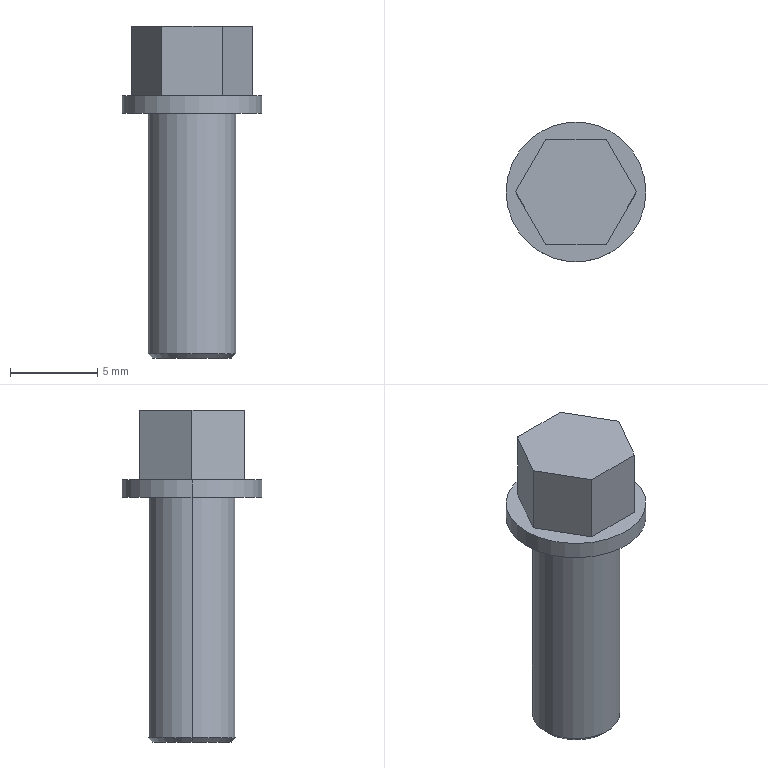Part | SolidWorks | features BaseBody 1 | 1 solid | 16 faces | box 8 x 8 x 19 mm | volume 449.388 mm3 | plane 10 | cylinder 4 | cone 2 | commonest cylinder face diameters 5 x2 8 x2
STEP:
#1=CARTESIAN_POINT('',(2.25,0.,-14.));
#2=VERTEX_POINT('',#1);
#3=CARTESIAN_POINT('',(-2.25,0.,-14.));
#4=VERTEX_POINT('',#3);
#5=CARTESIAN_POINT('',(0.,0.,-14.));
#6=DIRECTION('',(0.,0.,1.));
#7=DIRECTION('',(1.,0.,0.));
#8=AXIS2_PLACEMENT_3D('',#5,#6,#7);
#9=CIRCLE('',#8,2.25);
#10=EDGE_CURVE('',#2,#4,#9,.T.);
#11=ORIENTED_EDGE('',*,*,#10,.T.);
#12=CARTESIAN_POINT('',(-2.5,0.,-13.75));
#13=VERTEX_POINT('',#12);
#14=CARTESIAN_POINT('',(-2.375,0.,-13.875));
#15=DIRECTION('',(-0.7071,0.,0.7071));
#16=VECTOR('',#15,1000.);
#17=LINE('',#14,#16);
#18=EDGE_CURVE('',#4,#13,#17,.T.);
#19=ORIENTED_EDGE('',*,*,#18,.T.);
#20=CARTESIAN_POINT('',(2.5,0.,-13.75));
#21=VERTEX_POINT('',#20);
#22=CARTESIAN_POINT('',(0.,0.,-13.75));
#23=DIRECTION('',(0.,0.,-1.));
#24=DIRECTION('',(1.,0.,0.));
#25=AXIS2_PLACEMENT_3D('',#22,#23,#24);
#26=CIRCLE('',#25,2.5);
#27=EDGE_CURVE('',#13,#21,#26,.T.);
#28=ORIENTED_EDGE('',*,*,#27,.T.);
#29=CARTESIAN_POINT('',(2.375,0.,-13.875));
#30=DIRECTION('',(0.7071,0.,0.7071));
#31=VECTOR('',#30,1000.);
#32=LINE('',#29,#31);
#33=EDGE_CURVE('',#2,#21,#32,.T.);
#34=ORIENTED_EDGE('',*,*,#33,.F.);
#35=EDGE_LOOP('',(#11,#19,#28,#34));
#36=FACE_OUTER_BOUND('',#35,.T.);
#37=CARTESIAN_POINT('',(0.,0.,-13.875));
#38=DIRECTION('',(0.,0.,1.));
#39=DIRECTION('',(1.,0.,0.));
#40=AXIS2_PLACEMENT_3D('',#37,#38,#39);
#41=CONICAL_SURFACE('',#40,2.375,0.7854);
#42=ADVANCED_FACE('',(#36),#41,.T.);
#43=ORIENTED_EDGE('',*,*,#27,.F.);
#44=CARTESIAN_POINT('',(-2.5,0.,0.));
#45=VERTEX_POINT('',#44);
#46=CARTESIAN_POINT('',(-2.5,0.,0.));
#47=DIRECTION('',(0.,0.,1.));
#48=VECTOR('',#47,1000.);
#49=LINE('',#46,#48);
#50=EDGE_CURVE('',#13,#45,#49,.T.);
#51=ORIENTED_EDGE('',*,*,#50,.T.);
#52=CARTESIAN_POINT('',(2.5,0.,0.));
#53=VERTEX_POINT('',#52);
#54=CARTESIAN_POINT('',(0.,0.,0.));
#55=DIRECTION('',(0.,0.,1.));
#56=DIRECTION('',(1.,0.,0.));
#57=AXIS2_PLACEMENT_3D('',#54,#55,#56);
#58=CIRCLE('',#57,2.5);
#59=EDGE_CURVE('',#53,#45,#58,.T.);
#60=ORIENTED_EDGE('',*,*,#59,.F.);
#61=CARTESIAN_POINT('',(2.5,0.,0.));
#62=DIRECTION('',(0.,0.,1.));
#63=VECTOR('',#62,1000.);
#64=LINE('',#61,#63);
#65=EDGE_CURVE('',#21,#53,#64,.T.);
#66=ORIENTED_EDGE('',*,*,#65,.F.);
#67=EDGE_LOOP('',(#43,#51,#60,#66));
#68=FACE_OUTER_BOUND('',#67,.T.);
#69=CARTESIAN_POINT('',(0.,0.,0.));
#70=DIRECTION('',(0.,0.,1.));
#71=DIRECTION('',(1.,0.,0.));
#72=AXIS2_PLACEMENT_3D('',#69,#70,#71);
#73=CYLINDRICAL_SURFACE('',#72,2.5);
#74=ADVANCED_FACE('',(#68),#73,.T.);
#75=CARTESIAN_POINT('',(4.,0.,1.));
#76=VERTEX_POINT('',#75);
#77=CARTESIAN_POINT('',(-4.,0.,1.));
#78=VERTEX_POINT('',#77);
#79=CARTESIAN_POINT('',(0.,0.,1.));
#80=DIRECTION('',(0.,0.,1.));
#81=DIRECTION('',(-1.,0.,0.));
#82=AXIS2_PLACEMENT_3D('',#79,#80,#81);
#83=CIRCLE('',#82,4.);
#84=EDGE_CURVE('',#76,#78,#83,.T.);
#85=ORIENTED_EDGE('',*,*,#84,.F.);
#86=CARTESIAN_POINT('',(4.,0.,0.));
#87=VERTEX_POINT('',#86);
#88=CARTESIAN_POINT('',(4.,0.,0.));
#89=DIRECTION('',(0.,0.,-1.));
#90=VECTOR('',#89,1000.);
#91=LINE('',#88,#90);
#92=EDGE_CURVE('',#76,#87,#91,.T.);
#93=ORIENTED_EDGE('',*,*,#92,.T.);
#94=CARTESIAN_POINT('',(-4.,0.,0.));
#95=VERTEX_POINT('',#94);
#96=CARTESIAN_POINT('',(0.,0.,0.));
#97=DIRECTION('',(0.,0.,-1.));
#98=DIRECTION('',(-1.,0.,0.));
#99=AXIS2_PLACEMENT_3D('',#96,#97,#98);
#100=CIRCLE('',#99,4.);
#101=EDGE_CURVE('',#95,#87,#100,.T.);
#102=ORIENTED_EDGE('',*,*,#101,.F.);
#103=CARTESIAN_POINT('',(-4.,0.,0.));
#104=DIRECTION('',(0.,0.,-1.));
#105=VECTOR('',#104,1000.);
#106=LINE('',#103,#105);
#107=EDGE_CURVE('',#78,#95,#106,.T.);
#108=ORIENTED_EDGE('',*,*,#107,.F.);
#109=EDGE_LOOP('',(#85,#93,#102,#108));
#110=FACE_OUTER_BOUND('',#109,.T.);
#111=CARTESIAN_POINT('',(0.,0.,0.));
#112=DIRECTION('',(0.,0.,-1.));
#113=DIRECTION('',(-1.,0.,0.));
#114=AXIS2_PLACEMENT_3D('',#111,#112,#113);
#115=CYLINDRICAL_SURFACE('',#114,4.);
#116=ADVANCED_FACE('',(#110),#115,.T.);
#117=ORIENTED_EDGE('',*,*,#10,.F.);
#118=CARTESIAN_POINT('',(0.,0.,-14.));
#119=DIRECTION('',(0.,0.,1.));
#120=DIRECTION('',(1.,0.,0.));
#121=AXIS2_PLACEMENT_3D('',#118,#119,#120);
#122=CIRCLE('',#121,2.25);
#123=EDGE_CURVE('',#4,#2,#122,.T.);
#124=ORIENTED_EDGE('',*,*,#123,.F.);
#125=EDGE_LOOP('',(#117,#124));
#126=FACE_OUTER_BOUND('',#125,.T.);
#127=CARTESIAN_POINT('',(0.,0.,-14.));
#128=DIRECTION('',(0.,0.,1.));
#129=DIRECTION('',(1.,0.,0.));
#130=AXIS2_PLACEMENT_3D('',#127,#128,#129);
#131=PLANE('',#130);
#132=ADVANCED_FACE('',(#126),#131,.F.);
#133=CARTESIAN_POINT('',(-1.732,-3.,1.));
#134=VERTEX_POINT('',#133);
#135=CARTESIAN_POINT('',(-3.464,0.,1.));
#136=VERTEX_POINT('',#135);
#137=CARTESIAN_POINT('',(-3.031,-0.75,1.));
#138=DIRECTION('',(-0.5,0.866,0.));
#139=VECTOR('',#138,1000.);
#140=LINE('',#137,#139);
#141=EDGE_CURVE('',#134,#136,#140,.T.);
#142=ORIENTED_EDGE('',*,*,#141,.F.);
#143=CARTESIAN_POINT('',(-1.732,-3.,5.));
#144=VERTEX_POINT('',#143);
#145=CARTESIAN_POINT('',(-1.732,-3.,1.));
#146=DIRECTION('',(0.,0.,1.));
#147=VECTOR('',#146,1000.);
#148=LINE('',#145,#147);
#149=EDGE_CURVE('',#134,#144,#148,.T.);
#150=ORIENTED_EDGE('',*,*,#149,.T.);
#151=CARTESIAN_POINT('',(-3.464,0.,5.));
#152=VERTEX_POINT('',#151);
#153=CARTESIAN_POINT('',(-1.732,-3.,5.));
#154=DIRECTION('',(0.5,-0.866,0.));
#155=VECTOR('',#154,1000.);
#156=LINE('',#153,#155);
#157=EDGE_CURVE('',#152,#144,#156,.T.);
#158=ORIENTED_EDGE('',*,*,#157,.F.);
#159=CARTESIAN_POINT('',(-3.464,0.,1.));
#160=DIRECTION('',(0.,0.,1.));
#161=VECTOR('',#160,1000.);
#162=LINE('',#159,#161);
#163=EDGE_CURVE('',#136,#152,#162,.T.);
#164=ORIENTED_EDGE('',*,*,#163,.F.);
#165=EDGE_LOOP('',(#142,#150,#158,#164));
#166=FACE_OUTER_BOUND('',#165,.T.);
#167=CARTESIAN_POINT('',(-3.464,0.,1.));
#168=DIRECTION('',(-0.866,-0.5,0.));
#169=DIRECTION('',(-0.5,0.866,0.));
#170=AXIS2_PLACEMENT_3D('',#167,#168,#169);
#171=PLANE('',#170);
#172=ADVANCED_FACE('',(#166),#171,.T.);
#173=CARTESIAN_POINT('',(-1.732,3.,1.));
#174=VERTEX_POINT('',#173);
#175=CARTESIAN_POINT('',(-2.165,2.25,1.));
#176=DIRECTION('',(0.5,0.866,0.));
#177=VECTOR('',#176,1000.);
#178=LINE('',#175,#177);
#179=EDGE_CURVE('',#136,#174,#178,.T.);
#180=ORIENTED_EDGE('',*,*,#179,.F.);
#181=ORIENTED_EDGE('',*,*,#163,.T.);
#182=CARTESIAN_POINT('',(-1.732,3.,5.));
#183=VERTEX_POINT('',#182);
#184=CARTESIAN_POINT('',(-3.464,0.,5.));
#185=DIRECTION('',(-0.5,-0.866,0.));
#186=VECTOR('',#185,1000.);
#187=LINE('',#184,#186);
#188=EDGE_CURVE('',#183,#152,#187,.T.);
#189=ORIENTED_EDGE('',*,*,#188,.F.);
#190=CARTESIAN_POINT('',(-1.732,3.,1.));
#191=DIRECTION('',(0.,0.,1.));
#192=VECTOR('',#191,1000.);
#193=LINE('',#190,#192);
#194=EDGE_CURVE('',#174,#183,#193,.T.);
#195=ORIENTED_EDGE('',*,*,#194,.F.);
#196=EDGE_LOOP('',(#180,#181,#189,#195));
#197=FACE_OUTER_BOUND('',#196,.T.);
#198=CARTESIAN_POINT('',(-1.732,3.,1.));
#199=DIRECTION('',(-0.866,0.5,0.));
#200=DIRECTION('',(0.,0.,1.));
#201=AXIS2_PLACEMENT_3D('',#198,#199,#200);
#202=PLANE('',#201);
#203=ADVANCED_FACE('',(#197),#202,.T.);
#204=CARTESIAN_POINT('',(1.732,3.,1.));
#205=VERTEX_POINT('',#204);
#206=CARTESIAN_POINT('',(0.866,3.,1.));
#207=DIRECTION('',(1.,0.,0.));
#208=VECTOR('',#207,1000.);
#209=LINE('',#206,#208);
#210=EDGE_CURVE('',#174,#205,#209,.T.);
#211=ORIENTED_EDGE('',*,*,#210,.F.);
#212=ORIENTED_EDGE('',*,*,#194,.T.);
#213=CARTESIAN_POINT('',(1.732,3.,5.));
#214=VERTEX_POINT('',#213);
#215=CARTESIAN_POINT('',(-1.732,3.,5.));
#216=DIRECTION('',(-1.,0.,0.));
#217=VECTOR('',#216,1000.);
#218=LINE('',#215,#217);
#219=EDGE_CURVE('',#214,#183,#218,.T.);
#220=ORIENTED_EDGE('',*,*,#219,.F.);
#221=CARTESIAN_POINT('',(1.732,3.,1.));
#222=DIRECTION('',(0.,0.,1.));
#223=VECTOR('',#222,1000.);
#224=LINE('',#221,#223);
#225=EDGE_CURVE('',#205,#214,#224,.T.);
#226=ORIENTED_EDGE('',*,*,#225,.F.);
#227=EDGE_LOOP('',(#211,#212,#220,#226));
#228=FACE_OUTER_BOUND('',#227,.T.);
#229=CARTESIAN_POINT('',(1.732,3.,1.));
#230=DIRECTION('',(0.,1.,0.));
#231=DIRECTION('',(1.,0.,0.));
#232=AXIS2_PLACEMENT_3D('',#229,#230,#231);
#233=PLANE('',#232);
#234=ADVANCED_FACE('',(#228),#233,.T.);
#235=CARTESIAN_POINT('',(3.464,0.,1.));
#236=VERTEX_POINT('',#235);
#237=CARTESIAN_POINT('',(3.031,0.75,1.));
#238=DIRECTION('',(0.5,-0.866,0.));
#239=VECTOR('',#238,1000.);
#240=LINE('',#237,#239);
#241=EDGE_CURVE('',#205,#236,#240,.T.);
#242=ORIENTED_EDGE('',*,*,#241,.F.);
#243=ORIENTED_EDGE('',*,*,#225,.T.);
#244=CARTESIAN_POINT('',(3.464,0.,5.));
#245=VERTEX_POINT('',#244);
#246=CARTESIAN_POINT('',(1.732,3.,5.));
#247=DIRECTION('',(-0.5,0.866,0.));
#248=VECTOR('',#247,1000.);
#249=LINE('',#246,#248);
#250=EDGE_CURVE('',#245,#214,#249,.T.);
#251=ORIENTED_EDGE('',*,*,#250,.F.);
#252=CARTESIAN_POINT('',(3.464,0.,1.));
#253=DIRECTION('',(0.,0.,1.));
#254=VECTOR('',#253,1000.);
#255=LINE('',#252,#254);
#256=EDGE_CURVE('',#236,#245,#255,.T.);
#257=ORIENTED_EDGE('',*,*,#256,.F.);
#258=EDGE_LOOP('',(#242,#243,#251,#257));
#259=FACE_OUTER_BOUND('',#258,.T.);
#260=CARTESIAN_POINT('',(3.464,0.,1.));
#261=DIRECTION('',(0.866,0.5,0.));
#262=DIRECTION('',(0.,0.,-1.));
#263=AXIS2_PLACEMENT_3D('',#260,#261,#262);
#264=PLANE('',#263);
#265=ADVANCED_FACE('',(#259),#264,.T.);
#266=CARTESIAN_POINT('',(1.732,-3.,1.));
#267=VERTEX_POINT('',#266);
#268=CARTESIAN_POINT('',(2.165,-2.25,1.));
#269=DIRECTION('',(-0.5,-0.866,0.));
#270=VECTOR('',#269,1000.);
#271=LINE('',#268,#270);
#272=EDGE_CURVE('',#236,#267,#271,.T.);
#273=ORIENTED_EDGE('',*,*,#272,.F.);
#274=ORIENTED_EDGE('',*,*,#256,.T.);
#275=CARTESIAN_POINT('',(1.732,-3.,5.));
#276=VERTEX_POINT('',#275);
#277=CARTESIAN_POINT('',(3.464,0.,5.));
#278=DIRECTION('',(0.5,0.866,0.));
#279=VECTOR('',#278,1000.);
#280=LINE('',#277,#279);
#281=EDGE_CURVE('',#276,#245,#280,.T.);
#282=ORIENTED_EDGE('',*,*,#281,.F.);
#283=CARTESIAN_POINT('',(1.732,-3.,1.));
#284=DIRECTION('',(0.,0.,1.));
#285=VECTOR('',#284,1000.);
#286=LINE('',#283,#285);
#287=EDGE_CURVE('',#267,#276,#286,.T.);
#288=ORIENTED_EDGE('',*,*,#287,.F.);
#289=EDGE_LOOP('',(#273,#274,#282,#288));
#290=FACE_OUTER_BOUND('',#289,.T.);
#291=CARTESIAN_POINT('',(1.732,-3.,1.));
#292=DIRECTION('',(0.866,-0.5,0.));
#293=DIRECTION('',(0.,0.,-1.));
#294=AXIS2_PLACEMENT_3D('',#291,#292,#293);
#295=PLANE('',#294);
#296=ADVANCED_FACE('',(#290),#295,.T.);
#297=CARTESIAN_POINT('',(-0.866,-3.,1.));
#298=DIRECTION('',(-1.,0.,0.));
#299=VECTOR('',#298,1000.);
#300=LINE('',#297,#299);
#301=EDGE_CURVE('',#267,#134,#300,.T.);
#302=ORIENTED_EDGE('',*,*,#301,.F.);
#303=ORIENTED_EDGE('',*,*,#287,.T.);
#304=CARTESIAN_POINT('',(1.732,-3.,5.));
#305=DIRECTION('',(1.,0.,0.));
#306=VECTOR('',#305,1000.);
#307=LINE('',#304,#306);
#308=EDGE_CURVE('',#144,#276,#307,.T.);
#309=ORIENTED_EDGE('',*,*,#308,.F.);
#310=ORIENTED_EDGE('',*,*,#149,.F.);
#311=EDGE_LOOP('',(#302,#303,#309,#310));
#312=FACE_OUTER_BOUND('',#311,.T.);
#313=CARTESIAN_POINT('',(-1.732,-3.,1.));
#314=DIRECTION('',(0.,-1.,0.));
#315=DIRECTION('',(-1.,0.,0.));
#316=AXIS2_PLACEMENT_3D('',#313,#314,#315);
#317=PLANE('',#316);
#318=ADVANCED_FACE('',(#312),#317,.T.);
#319=ORIENTED_EDGE('',*,*,#308,.T.);
#320=ORIENTED_EDGE('',*,*,#281,.T.);
#321=ORIENTED_EDGE('',*,*,#250,.T.);
#322=ORIENTED_EDGE('',*,*,#219,.T.);
#323=ORIENTED_EDGE('',*,*,#188,.T.);
#324=ORIENTED_EDGE('',*,*,#157,.T.);
#325=EDGE_LOOP('',(#319,#320,#321,#322,#323,#324));
#326=FACE_OUTER_BOUND('',#325,.T.);
#327=CARTESIAN_POINT('',(0.,0.,5.));
#328=DIRECTION('',(0.,0.,1.));
#329=DIRECTION('',(1.,0.,0.));
#330=AXIS2_PLACEMENT_3D('',#327,#328,#329);
#331=PLANE('',#330);
#332=ADVANCED_FACE('',(#326),#331,.T.);
#333=ORIENTED_EDGE('',*,*,#59,.T.);
#334=CARTESIAN_POINT('',(0.,0.,0.));
#335=DIRECTION('',(0.,0.,1.));
#336=DIRECTION('',(1.,0.,0.));
#337=AXIS2_PLACEMENT_3D('',#334,#335,#336);
#338=CIRCLE('',#337,2.5);
#339=EDGE_CURVE('',#45,#53,#338,.T.);
#340=ORIENTED_EDGE('',*,*,#339,.T.);
#341=EDGE_LOOP('',(#333,#340));
#342=FACE_BOUND('',#341,.T.);
#343=ORIENTED_EDGE('',*,*,#101,.T.);
#344=CARTESIAN_POINT('',(0.,0.,0.));
#345=DIRECTION('',(0.,0.,-1.));
#346=DIRECTION('',(-1.,0.,0.));
#347=AXIS2_PLACEMENT_3D('',#344,#345,#346);
#348=CIRCLE('',#347,4.);
#349=EDGE_CURVE('',#87,#95,#348,.T.);
#350=ORIENTED_EDGE('',*,*,#349,.T.);
#351=EDGE_LOOP('',(#343,#350));
#352=FACE_OUTER_BOUND('',#351,.T.);
#353=CARTESIAN_POINT('',(0.,0.,0.));
#354=DIRECTION('',(0.,0.,1.));
#355=DIRECTION('',(1.,0.,0.));
#356=AXIS2_PLACEMENT_3D('',#353,#354,#355);
#357=PLANE('',#356);
#358=ADVANCED_FACE('',(#342,#352),#357,.F.);
#359=ORIENTED_EDGE('',*,*,#141,.T.);
#360=ORIENTED_EDGE('',*,*,#179,.T.);
#361=ORIENTED_EDGE('',*,*,#210,.T.);
#362=ORIENTED_EDGE('',*,*,#241,.T.);
#363=ORIENTED_EDGE('',*,*,#272,.T.);
#364=ORIENTED_EDGE('',*,*,#301,.T.);
#365=EDGE_LOOP('',(#359,#360,#361,#362,#363,#364));
#366=FACE_BOUND('',#365,.T.);
#367=CARTESIAN_POINT('',(0.,0.,1.));
#368=DIRECTION('',(0.,0.,1.));
#369=DIRECTION('',(-1.,0.,0.));
#370=AXIS2_PLACEMENT_3D('',#367,#368,#369);
#371=CIRCLE('',#370,4.);
#372=EDGE_CURVE('',#78,#76,#371,.T.);
#373=ORIENTED_EDGE('',*,*,#372,.T.);
#374=ORIENTED_EDGE('',*,*,#84,.T.);
#375=EDGE_LOOP('',(#373,#374));
#376=FACE_OUTER_BOUND('',#375,.T.);
#377=CARTESIAN_POINT('',(0.,0.,1.));
#378=DIRECTION('',(0.,0.,1.));
#379=DIRECTION('',(1.,0.,0.));
#380=AXIS2_PLACEMENT_3D('',#377,#378,#379);
#381=PLANE('',#380);
#382=ADVANCED_FACE('',(#366,#376),#381,.T.);
#383=ORIENTED_EDGE('',*,*,#92,.F.);
#384=ORIENTED_EDGE('',*,*,#372,.F.);
#385=ORIENTED_EDGE('',*,*,#107,.T.);
#386=ORIENTED_EDGE('',*,*,#349,.F.);
#387=EDGE_LOOP('',(#383,#384,#385,#386));
#388=FACE_OUTER_BOUND('',#387,.T.);
#389=CARTESIAN_POINT('',(0.,0.,0.));
#390=DIRECTION('',(0.,0.,-1.));
#391=DIRECTION('',(-1.,0.,0.));
#392=AXIS2_PLACEMENT_3D('',#389,#390,#391);
#393=CYLINDRICAL_SURFACE('',#392,4.);
#394=ADVANCED_FACE('',(#388),#393,.T.);
#395=ORIENTED_EDGE('',*,*,#50,.F.);
#396=CARTESIAN_POINT('',(0.,0.,-13.75));
#397=DIRECTION('',(0.,0.,-1.));
#398=DIRECTION('',(1.,0.,0.));
#399=AXIS2_PLACEMENT_3D('',#396,#397,#398);
#400=CIRCLE('',#399,2.5);
#401=EDGE_CURVE('',#21,#13,#400,.T.);
#402=ORIENTED_EDGE('',*,*,#401,.F.);
#403=ORIENTED_EDGE('',*,*,#65,.T.);
#404=ORIENTED_EDGE('',*,*,#339,.F.);
#405=EDGE_LOOP('',(#395,#402,#403,#404));
#406=FACE_OUTER_BOUND('',#405,.T.);
#407=CARTESIAN_POINT('',(0.,0.,0.));
#408=DIRECTION('',(0.,0.,1.));
#409=DIRECTION('',(1.,0.,0.));
#410=AXIS2_PLACEMENT_3D('',#407,#408,#409);
#411=CYLINDRICAL_SURFACE('',#410,2.5);
#412=ADVANCED_FACE('',(#406),#411,.T.);
#413=ORIENTED_EDGE('',*,*,#18,.F.);
#414=ORIENTED_EDGE('',*,*,#123,.T.);
#415=ORIENTED_EDGE('',*,*,#33,.T.);
#416=ORIENTED_EDGE('',*,*,#401,.T.);
#417=EDGE_LOOP('',(#413,#414,#415,#416));
#418=FACE_OUTER_BOUND('',#417,.T.);
#419=CARTESIAN_POINT('',(0.,0.,-13.875));
#420=DIRECTION('',(0.,0.,1.));
#421=DIRECTION('',(1.,0.,0.));
#422=AXIS2_PLACEMENT_3D('',#419,#420,#421);
#423=CONICAL_SURFACE('',#422,2.375,0.7854);
#424=ADVANCED_FACE('',(#418),#423,.T.);
#425=CLOSED_SHELL('',(#42,#74,#116,#132,#172,#203,#234,#265,#296,#318,#332,#358,#382,#394,#412,#424));
#426=MANIFOLD_SOLID_BREP('',#425);
#427=CARTESIAN_POINT('',(0.,0.,0.));
#428=DIRECTION('',(0.,0.,1.));
#429=DIRECTION('',(1.,0.,0.));
#430=AXIS2_PLACEMENT_3D('',#427,#428,#429);
#431=(LENGTH_UNIT()NAMED_UNIT(*)SI_UNIT(.MILLI.,.METRE.));
#432=UNCERTAINTY_MEASURE_WITH_UNIT(LENGTH_MEASURE(0.00001),#431,'','');
#433=(NAMED_UNIT(*)PLANE_ANGLE_UNIT()SI_UNIT($,.RADIAN.));
#434=(NAMED_UNIT(*)SI_UNIT($,.STERADIAN.)SOLID_ANGLE_UNIT());
#435=(GEOMETRIC_REPRESENTATION_CONTEXT(3)GLOBAL_UNCERTAINTY_ASSIGNED_CONTEXT((#432))GLOBAL_UNIT_ASSIGNED_CONTEXT((#431,#433,#434))REPRESENTATION_CONTEXT('',''));
#436=ADVANCED_BREP_SHAPE_REPRESENTATION('',(#426,#430),#435);